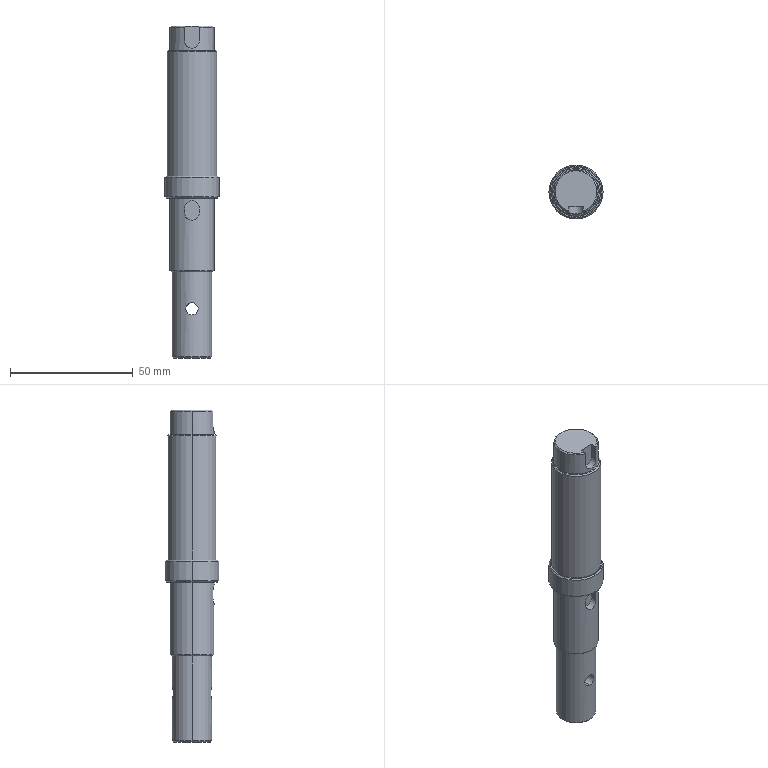Part | SolidWorks | features ICE 9, Chamfer 2, Extrusion 1 | 1 solid | 41 faces | box 22 x 22 x 135 mm | volume 36047 mm3 | cylinder 16 | cone 13 | plane 12 | commonest cylinder face diameters 6 x4 18 x4 5 x2 16 x2 20 x2 22 x2
STEP:
#1=CARTESIAN_POINT('',(0.,-8.,-52.));
#2=VERTEX_POINT('',#1);
#3=CARTESIAN_POINT('',(0.,-8.,-47.));
#4=VERTEX_POINT('',#3);
#5=CARTESIAN_POINT('',(0.,-8.,-52.));
#6=CARTESIAN_POINT('',(-0.1638,-8.,-52.));
#7=CARTESIAN_POINT('',(-0.3284,-7.995,-51.984));
#8=CARTESIAN_POINT('',(-0.6528,-7.975,-51.919));
#9=CARTESIAN_POINT('',(-0.8091,-7.96,-51.871));
#10=CARTESIAN_POINT('',(-1.111,-7.924,-51.746));
#11=CARTESIAN_POINT('',(-1.257,-7.902,-51.667));
#12=CARTESIAN_POINT('',(-1.527,-7.854,-51.486));
#13=CARTESIAN_POINT('',(-1.652,-7.828,-51.383));
#14=CARTESIAN_POINT('',(-1.883,-7.776,-51.152));
#15=CARTESIAN_POINT('',(-1.987,-7.75,-51.025));
#16=CARTESIAN_POINT('',(-2.168,-7.701,-50.756));
#17=CARTESIAN_POINT('',(-2.245,-7.679,-50.612));
#18=CARTESIAN_POINT('',(-2.372,-7.641,-50.308));
#19=CARTESIAN_POINT('',(-2.419,-7.626,-50.152));
#20=CARTESIAN_POINT('',(-2.483,-7.605,-49.831));
#21=CARTESIAN_POINT('',(-2.5,-7.599,-49.665));
#22=CARTESIAN_POINT('',(-2.5,-7.599,-49.335));
#23=CARTESIAN_POINT('',(-2.484,-7.605,-49.172));
#24=CARTESIAN_POINT('',(-2.42,-7.625,-48.85));
#25=CARTESIAN_POINT('',(-2.371,-7.641,-48.691));
#26=CARTESIAN_POINT('',(-2.183,-7.697,-48.239));
#27=CARTESIAN_POINT('',(-1.997,-7.75,-47.962));
#28=CARTESIAN_POINT('',(-1.654,-7.828,-47.618));
#29=CARTESIAN_POINT('',(-1.526,-7.854,-47.513));
#30=CARTESIAN_POINT('',(-1.256,-7.902,-47.332));
#31=CARTESIAN_POINT('',(-1.113,-7.924,-47.255));
#32=CARTESIAN_POINT('',(-0.8108,-7.96,-47.129));
#33=CARTESIAN_POINT('',(-0.6512,-7.975,-47.081));
#34=CARTESIAN_POINT('',(-0.3297,-7.995,-47.016));
#35=CARTESIAN_POINT('',(-0.1663,-8.,-47.));
#36=CARTESIAN_POINT('',(0.,-8.,-47.));
#37=B_SPLINE_CURVE_WITH_KNOTS('',3,(#5,#6,#7,#8,#9,#10,#11,#12,#13,#14,#15,#16,#17,#18,#19,#20,#21,#22,#23,#24,#25,#26,#27,#28,#29,#30,#31,#32,#33,#34,#35,#36),.UNSPECIFIED.,.F.,.F.,(4,2,2,2,2,2,2,2,2,2,2,2,2,2,2,4),(0.007866,0.008357,0.008849,0.00934,0.009832,0.01032,0.01081,0.01131,0.0118,0.01229,0.01278,0.01376,0.01425,0.01475,0.01524,0.01573),.UNSPECIFIED.);
#38=EDGE_CURVE('',#2,#4,#37,.T.);
#39=ORIENTED_EDGE('',*,*,#38,.F.);
#40=CARTESIAN_POINT('',(0.,8.,-52.));
#41=VERTEX_POINT('',#40);
#42=CARTESIAN_POINT('',(0.,-15.,-52.));
#43=DIRECTION('',(0.,1.,0.));
#44=VECTOR('',#43,1000.);
#45=LINE('',#42,#44);
#46=EDGE_CURVE('',#2,#41,#45,.T.);
#47=ORIENTED_EDGE('',*,*,#46,.T.);
#48=CARTESIAN_POINT('',(0.,8.,-47.));
#49=VERTEX_POINT('',#48);
#50=CARTESIAN_POINT('',(0.,8.,-47.));
#51=CARTESIAN_POINT('',(-0.1663,8.,-47.));
#52=CARTESIAN_POINT('',(-0.3296,7.995,-47.016));
#53=CARTESIAN_POINT('',(-0.6506,7.975,-47.081));
#54=CARTESIAN_POINT('',(-0.81,7.96,-47.129));
#55=CARTESIAN_POINT('',(-1.112,7.924,-47.255));
#56=CARTESIAN_POINT('',(-1.256,7.902,-47.332));
#57=CARTESIAN_POINT('',(-1.527,7.854,-47.513));
#58=CARTESIAN_POINT('',(-1.654,7.828,-47.618));
#59=CARTESIAN_POINT('',(-1.997,7.75,-47.962));
#60=CARTESIAN_POINT('',(-2.183,7.697,-48.239));
#61=CARTESIAN_POINT('',(-2.371,7.641,-48.69));
#62=CARTESIAN_POINT('',(-2.419,7.626,-48.848));
#63=CARTESIAN_POINT('',(-2.484,7.605,-49.172));
#64=CARTESIAN_POINT('',(-2.5,7.599,-49.335));
#65=CARTESIAN_POINT('',(-2.5,7.599,-49.663));
#66=CARTESIAN_POINT('',(-2.484,7.605,-49.83));
#67=CARTESIAN_POINT('',(-2.419,7.626,-50.151));
#68=CARTESIAN_POINT('',(-2.372,7.641,-50.308));
#69=CARTESIAN_POINT('',(-2.245,7.679,-50.612));
#70=CARTESIAN_POINT('',(-2.168,7.701,-50.756));
#71=CARTESIAN_POINT('',(-1.987,7.75,-51.026));
#72=CARTESIAN_POINT('',(-1.882,7.776,-51.153));
#73=CARTESIAN_POINT('',(-1.652,7.828,-51.384));
#74=CARTESIAN_POINT('',(-1.527,7.854,-51.486));
#75=CARTESIAN_POINT('',(-1.257,7.902,-51.667));
#76=CARTESIAN_POINT('',(-1.11,7.924,-51.746));
#77=CARTESIAN_POINT('',(-0.8089,7.96,-51.871));
#78=CARTESIAN_POINT('',(-0.6529,7.975,-51.919));
#79=CARTESIAN_POINT('',(-0.3297,7.995,-51.984));
#80=CARTESIAN_POINT('',(-0.1639,8.,-52.));
#81=CARTESIAN_POINT('',(0.,8.,-52.));
#82=B_SPLINE_CURVE_WITH_KNOTS('',3,(#50,#51,#52,#53,#54,#55,#56,#57,#58,#59,#60,#61,#62,#63,#64,#65,#66,#67,#68,#69,#70,#71,#72,#73,#74,#75,#76,#77,#78,#79,#80,#81),.UNSPECIFIED.,.F.,.F.,(4,2,2,2,2,2,2,2,2,2,2,2,2,2,2,4),(0.,0.0004916,0.0009832,0.001475,0.001966,0.00295,0.003441,0.003933,0.004424,0.004916,0.005408,0.005899,0.006391,0.006883,0.007374,0.007866),.UNSPECIFIED.);
#83=EDGE_CURVE('',#49,#41,#82,.T.);
#84=ORIENTED_EDGE('',*,*,#83,.F.);
#85=CARTESIAN_POINT('',(0.,-15.,-47.));
#86=DIRECTION('',(0.,1.,0.));
#87=VECTOR('',#86,1000.);
#88=LINE('',#85,#87);
#89=EDGE_CURVE('',#4,#49,#88,.T.);
#90=ORIENTED_EDGE('',*,*,#89,.F.);
#91=EDGE_LOOP('',(#39,#47,#84,#90));
#92=FACE_OUTER_BOUND('',#91,.T.);
#93=CARTESIAN_POINT('',(0.,-15.,-49.5));
#94=DIRECTION('',(0.,1.,0.));
#95=DIRECTION('',(0.,0.,1.));
#96=AXIS2_PLACEMENT_3D('',#93,#94,#95);
#97=CYLINDRICAL_SURFACE('',#96,2.5);
#98=ADVANCED_FACE('',(#92),#97,.F.);
#99=CARTESIAN_POINT('',(-7.5,0.,-69.5));
#100=VERTEX_POINT('',#99);
#101=CARTESIAN_POINT('',(7.5,0.,-69.5));
#102=VERTEX_POINT('',#101);
#103=CARTESIAN_POINT('',(0.,0.,-69.5));
#104=DIRECTION('',(0.,0.,-1.));
#105=DIRECTION('',(-1.,0.,0.));
#106=AXIS2_PLACEMENT_3D('',#103,#104,#105);
#107=CIRCLE('',#106,7.5);
#108=EDGE_CURVE('',#100,#102,#107,.T.);
#109=ORIENTED_EDGE('',*,*,#108,.F.);
#110=CARTESIAN_POINT('',(-8.,0.,-69.));
#111=VERTEX_POINT('',#110);
#112=CARTESIAN_POINT('',(-7.5,0.,-69.5));
#113=DIRECTION('',(-0.7071,0.,0.7071));
#114=VECTOR('',#113,1000.);
#115=LINE('',#112,#114);
#116=EDGE_CURVE('',#100,#111,#115,.T.);
#117=ORIENTED_EDGE('',*,*,#116,.T.);
#118=CARTESIAN_POINT('',(8.,0.,-69.));
#119=VERTEX_POINT('',#118);
#120=CARTESIAN_POINT('',(0.,0.,-69.));
#121=DIRECTION('',(0.,0.,1.));
#122=DIRECTION('',(-1.,0.,0.));
#123=AXIS2_PLACEMENT_3D('',#120,#121,#122);
#124=CIRCLE('',#123,8.);
#125=EDGE_CURVE('',#119,#111,#124,.T.);
#126=ORIENTED_EDGE('',*,*,#125,.F.);
#127=CARTESIAN_POINT('',(7.5,0.,-69.5));
#128=DIRECTION('',(0.7071,0.,0.7071));
#129=VECTOR('',#128,1000.);
#130=LINE('',#127,#129);
#131=EDGE_CURVE('',#102,#119,#130,.T.);
#132=ORIENTED_EDGE('',*,*,#131,.F.);
#133=EDGE_LOOP('',(#109,#117,#126,#132));
#134=FACE_OUTER_BOUND('',#133,.T.);
#135=CARTESIAN_POINT('',(0.,0.,-69.5));
#136=DIRECTION('',(0.,0.,1.));
#137=DIRECTION('',(1.,0.,0.));
#138=AXIS2_PLACEMENT_3D('',#135,#136,#137);
#139=CONICAL_SURFACE('',#138,7.5,0.7854);
#140=ADVANCED_FACE('',(#134),#139,.T.);
#141=ORIENTED_EDGE('',*,*,#83,.T.);
#142=CARTESIAN_POINT('',(0.,8.,-52.));
#143=CARTESIAN_POINT('',(0.1638,8.,-52.));
#144=CARTESIAN_POINT('',(0.3284,7.995,-51.984));
#145=CARTESIAN_POINT('',(0.6528,7.975,-51.919));
#146=CARTESIAN_POINT('',(0.8091,7.96,-51.871));
#147=CARTESIAN_POINT('',(1.111,7.924,-51.746));
#148=CARTESIAN_POINT('',(1.257,7.902,-51.667));
#149=CARTESIAN_POINT('',(1.527,7.854,-51.486));
#150=CARTESIAN_POINT('',(1.652,7.828,-51.383));
#151=CARTESIAN_POINT('',(1.883,7.776,-51.152));
#152=CARTESIAN_POINT('',(1.987,7.75,-51.025));
#153=CARTESIAN_POINT('',(2.168,7.701,-50.756));
#154=CARTESIAN_POINT('',(2.245,7.679,-50.612));
#155=CARTESIAN_POINT('',(2.372,7.641,-50.308));
#156=CARTESIAN_POINT('',(2.419,7.626,-50.152));
#157=CARTESIAN_POINT('',(2.483,7.605,-49.831));
#158=CARTESIAN_POINT('',(2.5,7.599,-49.665));
#159=CARTESIAN_POINT('',(2.5,7.599,-49.335));
#160=CARTESIAN_POINT('',(2.484,7.605,-49.172));
#161=CARTESIAN_POINT('',(2.42,7.625,-48.85));
#162=CARTESIAN_POINT('',(2.371,7.641,-48.691));
#163=CARTESIAN_POINT('',(2.183,7.697,-48.239));
#164=CARTESIAN_POINT('',(1.997,7.75,-47.962));
#165=CARTESIAN_POINT('',(1.654,7.828,-47.618));
#166=CARTESIAN_POINT('',(1.526,7.854,-47.513));
#167=CARTESIAN_POINT('',(1.256,7.902,-47.332));
#168=CARTESIAN_POINT('',(1.113,7.924,-47.255));
#169=CARTESIAN_POINT('',(0.8108,7.96,-47.129));
#170=CARTESIAN_POINT('',(0.6512,7.975,-47.081));
#171=CARTESIAN_POINT('',(0.3297,7.995,-47.016));
#172=CARTESIAN_POINT('',(0.1663,8.,-47.));
#173=CARTESIAN_POINT('',(0.,8.,-47.));
#174=B_SPLINE_CURVE_WITH_KNOTS('',3,(#142,#143,#144,#145,#146,#147,#148,#149,#150,#151,#152,#153,#154,#155,#156,#157,#158,#159,#160,#161,#162,#163,#164,#165,#166,#167,#168,#169,#170,#171,#172,#173),.UNSPECIFIED.,.F.,.F.,(4,2,2,2,2,2,2,2,2,2,2,2,2,2,2,4),(0.007866,0.008357,0.008849,0.00934,0.009832,0.01032,0.01081,0.01131,0.0118,0.01229,0.01278,0.01376,0.01425,0.01475,0.01524,0.01573),.UNSPECIFIED.);
#175=EDGE_CURVE('',#41,#49,#174,.T.);
#176=ORIENTED_EDGE('',*,*,#175,.T.);
#177=EDGE_LOOP('',(#141,#176));
#178=FACE_BOUND('',#177,.T.);
#179=ORIENTED_EDGE('',*,*,#125,.T.);
#180=CARTESIAN_POINT('',(-8.,0.,-34.5));
#181=VERTEX_POINT('',#180);
#182=CARTESIAN_POINT('',(-8.,0.,-69.5));
#183=DIRECTION('',(0.,0.,1.));
#184=VECTOR('',#183,1000.);
#185=LINE('',#182,#184);
#186=EDGE_CURVE('',#111,#181,#185,.T.);
#187=ORIENTED_EDGE('',*,*,#186,.T.);
#188=CARTESIAN_POINT('',(8.,0.,-34.5));
#189=VERTEX_POINT('',#188);
#190=CARTESIAN_POINT('',(0.,0.,-34.5));
#191=DIRECTION('',(0.,0.,-1.));
#192=DIRECTION('',(-1.,0.,0.));
#193=AXIS2_PLACEMENT_3D('',#190,#191,#192);
#194=CIRCLE('',#193,8.);
#195=EDGE_CURVE('',#181,#189,#194,.T.);
#196=ORIENTED_EDGE('',*,*,#195,.T.);
#197=CARTESIAN_POINT('',(8.,0.,-69.5));
#198=DIRECTION('',(0.,0.,1.));
#199=VECTOR('',#198,1000.);
#200=LINE('',#197,#199);
#201=EDGE_CURVE('',#119,#189,#200,.T.);
#202=ORIENTED_EDGE('',*,*,#201,.F.);
#203=EDGE_LOOP('',(#179,#187,#196,#202));
#204=FACE_OUTER_BOUND('',#203,.T.);
#205=CARTESIAN_POINT('',(0.,0.,-69.5));
#206=DIRECTION('',(0.,0.,1.));
#207=DIRECTION('',(1.,0.,0.));
#208=AXIS2_PLACEMENT_3D('',#205,#206,#207);
#209=CYLINDRICAL_SURFACE('',#208,8.);
#210=ADVANCED_FACE('',(#178,#204),#209,.T.);
#211=CARTESIAN_POINT('',(8.5,0.,65.5));
#212=VERTEX_POINT('',#211);
#213=CARTESIAN_POINT('',(-8.5,0.,65.5));
#214=VERTEX_POINT('',#213);
#215=CARTESIAN_POINT('',(0.,0.,65.5));
#216=DIRECTION('',(0.,0.,1.));
#217=DIRECTION('',(1.,0.,0.));
#218=AXIS2_PLACEMENT_3D('',#215,#216,#217);
#219=CIRCLE('',#218,8.5);
#220=EDGE_CURVE('',#212,#214,#219,.T.);
#221=ORIENTED_EDGE('',*,*,#220,.F.);
#222=CARTESIAN_POINT('',(9.,0.,65.));
#223=VERTEX_POINT('',#222);
#224=CARTESIAN_POINT('',(8.5,0.,65.5));
#225=DIRECTION('',(0.7071,0.,-0.7071));
#226=VECTOR('',#225,1000.);
#227=LINE('',#224,#226);
#228=EDGE_CURVE('',#212,#223,#227,.T.);
#229=ORIENTED_EDGE('',*,*,#228,.T.);
#230=CARTESIAN_POINT('',(-9.,0.,65.));
#231=VERTEX_POINT('',#230);
#232=CARTESIAN_POINT('',(0.,0.,65.));
#233=DIRECTION('',(0.,0.,-1.));
#234=DIRECTION('',(1.,0.,0.));
#235=AXIS2_PLACEMENT_3D('',#232,#233,#234);
#236=CIRCLE('',#235,9.);
#237=EDGE_CURVE('',#231,#223,#236,.T.);
#238=ORIENTED_EDGE('',*,*,#237,.F.);
#239=CARTESIAN_POINT('',(-8.5,0.,65.5));
#240=DIRECTION('',(-0.7071,0.,-0.7071));
#241=VECTOR('',#240,1000.);
#242=LINE('',#239,#241);
#243=EDGE_CURVE('',#214,#231,#242,.T.);
#244=ORIENTED_EDGE('',*,*,#243,.F.);
#245=EDGE_LOOP('',(#221,#229,#238,#244));
#246=FACE_OUTER_BOUND('',#245,.T.);
#247=CARTESIAN_POINT('',(0.,0.,65.5));
#248=DIRECTION('',(0.,0.,-1.));
#249=DIRECTION('',(-1.,0.,0.));
#250=AXIS2_PLACEMENT_3D('',#247,#248,#249);
#251=CONICAL_SURFACE('',#250,8.5,0.7854);
#252=ADVANCED_FACE('',(#246),#251,.T.);
#253=CARTESIAN_POINT('',(-3.,-7.953,65.5));
#254=VERTEX_POINT('',#253);
#255=CARTESIAN_POINT('',(0.,0.,65.5));
#256=DIRECTION('',(0.,0.,1.));
#257=DIRECTION('',(1.,0.,0.));
#258=AXIS2_PLACEMENT_3D('',#255,#256,#257);
#259=CIRCLE('',#258,8.5);
#260=EDGE_CURVE('',#214,#254,#259,.T.);
#261=ORIENTED_EDGE('',*,*,#260,.F.);
#262=ORIENTED_EDGE('',*,*,#243,.T.);
#263=CARTESIAN_POINT('',(-3.,-8.485,65.));
#264=VERTEX_POINT('',#263);
#265=CARTESIAN_POINT('',(0.,0.,65.));
#266=DIRECTION('',(0.,0.,-1.));
#267=DIRECTION('',(1.,0.,0.));
#268=AXIS2_PLACEMENT_3D('',#265,#266,#267);
#269=CIRCLE('',#268,9.);
#270=EDGE_CURVE('',#264,#231,#269,.T.);
#271=ORIENTED_EDGE('',*,*,#270,.F.);
#272=CARTESIAN_POINT('',(-3.,-7.953,65.5));
#273=CARTESIAN_POINT('',(-3.,-8.131,65.334));
#274=CARTESIAN_POINT('',(-3.,-8.308,65.167));
#275=CARTESIAN_POINT('',(-3.,-8.485,65.));
#276=B_SPLINE_CURVE_WITH_KNOTS('',3,(#272,#273,#274,#275),.UNSPECIFIED.,.F.,.F.,(4,4),(0.,0.0007303),.UNSPECIFIED.);
#277=EDGE_CURVE('',#254,#264,#276,.T.);
#278=ORIENTED_EDGE('',*,*,#277,.F.);
#279=EDGE_LOOP('',(#261,#262,#271,#278));
#280=FACE_OUTER_BOUND('',#279,.T.);
#281=CARTESIAN_POINT('',(0.,0.,65.5));
#282=DIRECTION('',(0.,0.,-1.));
#283=DIRECTION('',(-1.,0.,0.));
#284=AXIS2_PLACEMENT_3D('',#281,#282,#283);
#285=CONICAL_SURFACE('',#284,8.5,0.7854);
#286=ADVANCED_FACE('',(#280),#285,.T.);
#287=CARTESIAN_POINT('',(9.5,0.,55.5));
#288=VERTEX_POINT('',#287);
#289=CARTESIAN_POINT('',(-9.5,0.,55.5));
#290=VERTEX_POINT('',#289);
#291=CARTESIAN_POINT('',(0.,0.,55.5));
#292=DIRECTION('',(0.,0.,1.));
#293=DIRECTION('',(1.,0.,0.));
#294=AXIS2_PLACEMENT_3D('',#291,#292,#293);
#295=CIRCLE('',#294,9.5);
#296=EDGE_CURVE('',#288,#290,#295,.T.);
#297=ORIENTED_EDGE('',*,*,#296,.F.);
#298=CARTESIAN_POINT('',(10.,0.,55.));
#299=VERTEX_POINT('',#298);
#300=CARTESIAN_POINT('',(9.5,0.,55.5));
#301=DIRECTION('',(0.7071,0.,-0.7071));
#302=VECTOR('',#301,1000.);
#303=LINE('',#300,#302);
#304=EDGE_CURVE('',#288,#299,#303,.T.);
#305=ORIENTED_EDGE('',*,*,#304,.T.);
#306=CARTESIAN_POINT('',(-10.,0.,55.));
#307=VERTEX_POINT('',#306);
#308=CARTESIAN_POINT('',(0.,0.,55.));
#309=DIRECTION('',(0.,0.,-1.));
#310=DIRECTION('',(1.,0.,0.));
#311=AXIS2_PLACEMENT_3D('',#308,#309,#310);
#312=CIRCLE('',#311,10.);
#313=EDGE_CURVE('',#307,#299,#312,.T.);
#314=ORIENTED_EDGE('',*,*,#313,.F.);
#315=CARTESIAN_POINT('',(-9.5,0.,55.5));
#316=DIRECTION('',(-0.7071,0.,-0.7071));
#317=VECTOR('',#316,1000.);
#318=LINE('',#315,#317);
#319=EDGE_CURVE('',#290,#307,#318,.T.);
#320=ORIENTED_EDGE('',*,*,#319,.F.);
#321=EDGE_LOOP('',(#297,#305,#314,#320));
#322=FACE_OUTER_BOUND('',#321,.T.);
#323=CARTESIAN_POINT('',(0.,0.,55.5));
#324=DIRECTION('',(0.,0.,-1.));
#325=DIRECTION('',(-1.,0.,0.));
#326=AXIS2_PLACEMENT_3D('',#323,#324,#325);
#327=CONICAL_SURFACE('',#326,9.5,0.7854);
#328=ADVANCED_FACE('',(#322),#327,.T.);
#329=CARTESIAN_POINT('',(10.5,0.,4.5));
#330=VERTEX_POINT('',#329);
#331=CARTESIAN_POINT('',(-10.5,0.,4.5));
#332=VERTEX_POINT('',#331);
#333=CARTESIAN_POINT('',(0.,0.,4.5));
#334=DIRECTION('',(0.,0.,1.));
#335=DIRECTION('',(1.,0.,0.));
#336=AXIS2_PLACEMENT_3D('',#333,#334,#335);
#337=CIRCLE('',#336,10.5);
#338=EDGE_CURVE('',#330,#332,#337,.T.);
#339=ORIENTED_EDGE('',*,*,#338,.F.);
#340=CARTESIAN_POINT('',(11.,0.,4.));
#341=VERTEX_POINT('',#340);
#342=CARTESIAN_POINT('',(10.5,0.,4.5));
#343=DIRECTION('',(0.7071,0.,-0.7071));
#344=VECTOR('',#343,1000.);
#345=LINE('',#342,#344);
#346=EDGE_CURVE('',#330,#341,#345,.T.);
#347=ORIENTED_EDGE('',*,*,#346,.T.);
#348=CARTESIAN_POINT('',(-11.,0.,4.));
#349=VERTEX_POINT('',#348);
#350=CARTESIAN_POINT('',(0.,0.,4.));
#351=DIRECTION('',(0.,0.,-1.));
#352=DIRECTION('',(1.,0.,0.));
#353=AXIS2_PLACEMENT_3D('',#350,#351,#352);
#354=CIRCLE('',#353,11.);
#355=EDGE_CURVE('',#349,#341,#354,.T.);
#356=ORIENTED_EDGE('',*,*,#355,.F.);
#357=CARTESIAN_POINT('',(-10.5,0.,4.5));
#358=DIRECTION('',(-0.7071,0.,-0.7071));
#359=VECTOR('',#358,1000.);
#360=LINE('',#357,#359);
#361=EDGE_CURVE('',#332,#349,#360,.T.);
#362=ORIENTED_EDGE('',*,*,#361,.F.);
#363=EDGE_LOOP('',(#339,#347,#356,#362));
#364=FACE_OUTER_BOUND('',#363,.T.);
#365=CARTESIAN_POINT('',(0.,0.,4.5));
#366=DIRECTION('',(0.,0.,-1.));
#367=DIRECTION('',(-1.,0.,0.));
#368=AXIS2_PLACEMENT_3D('',#365,#366,#367);
#369=CONICAL_SURFACE('',#368,10.5,0.7854);
#370=ADVANCED_FACE('',(#364),#369,.T.);
#371=CARTESIAN_POINT('',(-10.5,0.,-4.5));
#372=VERTEX_POINT('',#371);
#373=CARTESIAN_POINT('',(10.5,0.,-4.5));
#374=VERTEX_POINT('',#373);
#375=CARTESIAN_POINT('',(0.,0.,-4.5));
#376=DIRECTION('',(0.,0.,-1.));
#377=DIRECTION('',(1.,0.,0.));
#378=AXIS2_PLACEMENT_3D('',#375,#376,#377);
#379=CIRCLE('',#378,10.5);
#380=EDGE_CURVE('',#372,#374,#379,.T.);
#381=ORIENTED_EDGE('',*,*,#380,.F.);
#382=CARTESIAN_POINT('',(-11.,0.,-4.));
#383=VERTEX_POINT('',#382);
#384=CARTESIAN_POINT('',(-11.,0.,-4.));
#385=DIRECTION('',(-0.7071,0.,0.7071));
#386=VECTOR('',#385,1000.);
#387=LINE('',#384,#386);
#388=EDGE_CURVE('',#372,#383,#387,.T.);
#389=ORIENTED_EDGE('',*,*,#388,.T.);
#390=CARTESIAN_POINT('',(11.,0.,-4.));
#391=VERTEX_POINT('',#390);
#392=CARTESIAN_POINT('',(0.,0.,-4.));
#393=DIRECTION('',(0.,0.,1.));
#394=DIRECTION('',(1.,0.,0.));
#395=AXIS2_PLACEMENT_3D('',#392,#393,#394);
#396=CIRCLE('',#395,11.);
#397=EDGE_CURVE('',#391,#383,#396,.T.);
#398=ORIENTED_EDGE('',*,*,#397,.F.);
#399=CARTESIAN_POINT('',(11.,0.,-4.));
#400=DIRECTION('',(0.7071,0.,0.7071));
#401=VECTOR('',#400,1000.);
#402=LINE('',#399,#401);
#403=EDGE_CURVE('',#374,#391,#402,.T.);
#404=ORIENTED_EDGE('',*,*,#403,.F.);
#405=EDGE_LOOP('',(#381,#389,#398,#404));
#406=FACE_OUTER_BOUND('',#405,.T.);
#407=CARTESIAN_POINT('',(0.,0.,-4.));
#408=DIRECTION('',(0.,0.,1.));
#409=DIRECTION('',(1.,0.,0.));
#410=AXIS2_PLACEMENT_3D('',#407,#408,#409);
#411=CONICAL_SURFACE('',#410,11.,0.7854);
#412=ADVANCED_FACE('',(#406),#411,.T.);
#413=CARTESIAN_POINT('',(-8.5,0.,-34.5));
#414=VERTEX_POINT('',#413);
#415=CARTESIAN_POINT('',(8.5,0.,-34.5));
#416=VERTEX_POINT('',#415);
#417=CARTESIAN_POINT('',(0.,0.,-34.5));
#418=DIRECTION('',(0.,0.,-1.));
#419=DIRECTION('',(-1.,0.,0.));
#420=AXIS2_PLACEMENT_3D('',#417,#418,#419);
#421=CIRCLE('',#420,8.5);
#422=EDGE_CURVE('',#414,#416,#421,.T.);
#423=ORIENTED_EDGE('',*,*,#422,.F.);
#424=CARTESIAN_POINT('',(-9.,0.,-34.));
#425=VERTEX_POINT('',#424);
#426=CARTESIAN_POINT('',(-8.5,0.,-34.5));
#427=DIRECTION('',(-0.7071,0.,0.7071));
#428=VECTOR('',#427,1000.);
#429=LINE('',#426,#428);
#430=EDGE_CURVE('',#414,#425,#429,.T.);
#431=ORIENTED_EDGE('',*,*,#430,.T.);
#432=CARTESIAN_POINT('',(9.,0.,-34.));
#433=VERTEX_POINT('',#432);
#434=CARTESIAN_POINT('',(0.,0.,-34.));
#435=DIRECTION('',(0.,0.,1.));
#436=DIRECTION('',(-1.,0.,0.));
#437=AXIS2_PLACEMENT_3D('',#434,#435,#436);
#438=CIRCLE('',#437,9.);
#439=EDGE_CURVE('',#433,#425,#438,.T.);
#440=ORIENTED_EDGE('',*,*,#439,.F.);
#441=CARTESIAN_POINT('',(8.5,0.,-34.5));
#442=DIRECTION('',(0.7071,0.,0.7071));
#443=VECTOR('',#442,1000.);
#444=LINE('',#441,#443);
#445=EDGE_CURVE('',#416,#433,#444,.T.);
#446=ORIENTED_EDGE('',*,*,#445,.F.);
#447=EDGE_LOOP('',(#423,#431,#440,#446));
#448=FACE_OUTER_BOUND('',#447,.T.);
#449=CARTESIAN_POINT('',(0.,0.,-34.5));
#450=DIRECTION('',(0.,0.,1.));
#451=DIRECTION('',(1.,0.,0.));
#452=AXIS2_PLACEMENT_3D('',#449,#450,#451);
#453=CONICAL_SURFACE('',#452,8.5,0.7854);
#454=ADVANCED_FACE('',(#448),#453,.T.);
#455=CARTESIAN_POINT('',(0.,-9.,-5.5));
#456=VERTEX_POINT('',#455);
#457=CARTESIAN_POINT('',(3.,-8.485,-8.5));
#458=VERTEX_POINT('',#457);
#459=CARTESIAN_POINT('',(0.,-9.,-5.5));
#460=CARTESIAN_POINT('',(0.1971,-9.,-5.5));
#461=CARTESIAN_POINT('',(0.3973,-8.993,-5.52));
#462=CARTESIAN_POINT('',(0.7829,-8.968,-5.597));
#463=CARTESIAN_POINT('',(0.9705,-8.949,-5.654));
#464=CARTESIAN_POINT('',(1.335,-8.902,-5.806));
#465=CARTESIAN_POINT('',(1.508,-8.874,-5.899));
#466=CARTESIAN_POINT('',(1.831,-8.813,-6.116));
#467=CARTESIAN_POINT('',(1.984,-8.78,-6.241));
#468=CARTESIAN_POINT('',(2.26,-8.713,-6.517));
#469=CARTESIAN_POINT('',(2.383,-8.68,-6.667));
#470=CARTESIAN_POINT('',(2.6,-8.617,-6.991));
#471=CARTESIAN_POINT('',(2.694,-8.588,-7.166));
#472=CARTESIAN_POINT('',(2.844,-8.539,-7.526));
#473=CARTESIAN_POINT('',(2.902,-8.519,-7.713));
#474=CARTESIAN_POINT('',(2.98,-8.492,-8.101));
#475=CARTESIAN_POINT('',(3.,-8.485,-8.3));
#476=CARTESIAN_POINT('',(3.,-8.485,-8.5));
#477=B_SPLINE_CURVE_WITH_KNOTS('',3,(#459,#460,#461,#462,#463,#464,#465,#466,#467,#468,#469,#470,#471,#472,#473,#474,#475,#476),.UNSPECIFIED.,.F.,.F.,(4,2,2,2,2,2,2,2,4),(0.004725,0.005315,0.005905,0.006494,0.007084,0.007674,0.008264,0.008854,0.009444),.UNSPECIFIED.);
#478=EDGE_CURVE('',#456,#458,#477,.T.);
#479=ORIENTED_EDGE('',*,*,#478,.F.);
#480=CARTESIAN_POINT('',(0.,-6.,-5.5));
#481=VERTEX_POINT('',#480);
#482=CARTESIAN_POINT('',(0.,-19.,-5.5));
#483=DIRECTION('',(0.,1.,0.));
#484=VECTOR('',#483,1000.);
#485=LINE('',#482,#484);
#486=EDGE_CURVE('',#456,#481,#485,.T.);
#487=ORIENTED_EDGE('',*,*,#486,.T.);
#488=CARTESIAN_POINT('',(3.,-6.,-8.5));
#489=VERTEX_POINT('',#488);
#490=CARTESIAN_POINT('',(0.,-6.,-8.5));
#491=DIRECTION('',(0.,-1.,0.));
#492=DIRECTION('',(0.,0.,-1.));
#493=AXIS2_PLACEMENT_3D('',#490,#491,#492);
#494=CIRCLE('',#493,3.);
#495=EDGE_CURVE('',#489,#481,#494,.T.);
#496=ORIENTED_EDGE('',*,*,#495,.F.);
#497=CARTESIAN_POINT('',(3.,-19.,-8.5));
#498=DIRECTION('',(0.,1.,0.));
#499=VECTOR('',#498,1000.);
#500=LINE('',#497,#499);
#501=EDGE_CURVE('',#458,#489,#500,.T.);
#502=ORIENTED_EDGE('',*,*,#501,.F.);
#503=EDGE_LOOP('',(#479,#487,#496,#502));
#504=FACE_OUTER_BOUND('',#503,.T.);
#505=CARTESIAN_POINT('',(0.,-19.,-8.5));
#506=DIRECTION('',(0.,1.,0.));
#507=DIRECTION('',(0.,0.,1.));
#508=AXIS2_PLACEMENT_3D('',#505,#506,#507);
#509=CYLINDRICAL_SURFACE('',#508,3.);
#510=ADVANCED_FACE('',(#504),#509,.F.);
#511=ORIENTED_EDGE('',*,*,#237,.T.);
#512=CARTESIAN_POINT('',(9.,0.,55.5));
#513=VERTEX_POINT('',#512);
#514=CARTESIAN_POINT('',(9.,0.,65.5));
#515=DIRECTION('',(0.,0.,-1.));
#516=VECTOR('',#515,1000.);
#517=LINE('',#514,#516);
#518=EDGE_CURVE('',#223,#513,#517,.T.);
#519=ORIENTED_EDGE('',*,*,#518,.T.);
#520=CARTESIAN_POINT('',(-9.,0.,55.5));
#521=VERTEX_POINT('',#520);
#522=CARTESIAN_POINT('',(0.,0.,55.5));
#523=DIRECTION('',(0.,0.,1.));
#524=DIRECTION('',(1.,0.,0.));
#525=AXIS2_PLACEMENT_3D('',#522,#523,#524);
#526=CIRCLE('',#525,9.);
#527=EDGE_CURVE('',#513,#521,#526,.T.);
#528=ORIENTED_EDGE('',*,*,#527,.T.);
#529=CARTESIAN_POINT('',(-9.,0.,65.5));
#530=DIRECTION('',(0.,0.,-1.));
#531=VECTOR('',#530,1000.);
#532=LINE('',#529,#531);
#533=EDGE_CURVE('',#231,#521,#532,.T.);
#534=ORIENTED_EDGE('',*,*,#533,.F.);
#535=EDGE_LOOP('',(#511,#519,#528,#534));
#536=FACE_OUTER_BOUND('',#535,.T.);
#537=CARTESIAN_POINT('',(0.,0.,65.5));
#538=DIRECTION('',(0.,0.,-1.));
#539=DIRECTION('',(-1.,0.,0.));
#540=AXIS2_PLACEMENT_3D('',#537,#538,#539);
#541=CYLINDRICAL_SURFACE('',#540,9.);
#542=ADVANCED_FACE('',(#536),#541,.T.);
#543=ORIENTED_EDGE('',*,*,#313,.T.);
#544=CARTESIAN_POINT('',(10.,0.,4.5));
#545=VERTEX_POINT('',#544);
#546=CARTESIAN_POINT('',(10.,0.,55.5));
#547=DIRECTION('',(0.,0.,-1.));
#548=VECTOR('',#547,1000.);
#549=LINE('',#546,#548);
#550=EDGE_CURVE('',#299,#545,#549,.T.);
#551=ORIENTED_EDGE('',*,*,#550,.T.);
#552=CARTESIAN_POINT('',(-10.,0.,4.5));
#553=VERTEX_POINT('',#552);
#554=CARTESIAN_POINT('',(0.,0.,4.5));
#555=DIRECTION('',(0.,0.,1.));
#556=DIRECTION('',(1.,0.,0.));
#557=AXIS2_PLACEMENT_3D('',#554,#555,#556);
#558=CIRCLE('',#557,10.);
#559=EDGE_CURVE('',#545,#553,#558,.T.);
#560=ORIENTED_EDGE('',*,*,#559,.T.);
#561=CARTESIAN_POINT('',(-10.,0.,55.5));
#562=DIRECTION('',(0.,0.,-1.));
#563=VECTOR('',#562,1000.);
#564=LINE('',#561,#563);
#565=EDGE_CURVE('',#307,#553,#564,.T.);
#566=ORIENTED_EDGE('',*,*,#565,.F.);
#567=EDGE_LOOP('',(#543,#551,#560,#566));
#568=FACE_OUTER_BOUND('',#567,.T.);
#569=CARTESIAN_POINT('',(0.,0.,55.5));
#570=DIRECTION('',(0.,0.,-1.));
#571=DIRECTION('',(-1.,0.,0.));
#572=AXIS2_PLACEMENT_3D('',#569,#570,#571);
#573=CYLINDRICAL_SURFACE('',#572,10.);
#574=ADVANCED_FACE('',(#568),#573,.T.);
#575=ORIENTED_EDGE('',*,*,#439,.T.);
#576=CARTESIAN_POINT('',(-9.,0.,-4.5));
#577=VERTEX_POINT('',#576);
#578=CARTESIAN_POINT('',(-9.,0.,-34.5));
#579=DIRECTION('',(0.,0.,1.));
#580=VECTOR('',#579,1000.);
#581=LINE('',#578,#580);
#582=EDGE_CURVE('',#425,#577,#581,.T.);
#583=ORIENTED_EDGE('',*,*,#582,.T.);
#584=CARTESIAN_POINT('',(9.,0.,-4.5));
#585=VERTEX_POINT('',#584);
#586=CARTESIAN_POINT('',(0.,0.,-4.5));
#587=DIRECTION('',(0.,0.,-1.));
#588=DIRECTION('',(1.,0.,0.));
#589=AXIS2_PLACEMENT_3D('',#586,#587,#588);
#590=CIRCLE('',#589,9.);
#591=EDGE_CURVE('',#577,#585,#590,.T.);
#592=ORIENTED_EDGE('',*,*,#591,.T.);
#593=CARTESIAN_POINT('',(9.,0.,-34.5));
#594=DIRECTION('',(0.,0.,1.));
#595=VECTOR('',#594,1000.);
#596=LINE('',#593,#595);
#597=EDGE_CURVE('',#433,#585,#596,.T.);
#598=ORIENTED_EDGE('',*,*,#597,.F.);
#599=EDGE_LOOP('',(#575,#583,#592,#598));
#600=FACE_OUTER_BOUND('',#599,.T.);
#601=CARTESIAN_POINT('',(0.,0.,-34.5));
#602=DIRECTION('',(0.,0.,1.));
#603=DIRECTION('',(1.,0.,0.));
#604=AXIS2_PLACEMENT_3D('',#601,#602,#603);
#605=CYLINDRICAL_SURFACE('',#604,9.);
#606=ADVANCED_FACE('',(#600),#605,.T.);
#607=ORIENTED_EDGE('',*,*,#355,.T.);
#608=CARTESIAN_POINT('',(11.,0.,4.5));
#609=DIRECTION('',(0.,0.,-1.));
#610=VECTOR('',#609,1000.);
#611=LINE('',#608,#610);
#612=EDGE_CURVE('',#341,#391,#611,.T.);
#613=ORIENTED_EDGE('',*,*,#612,.T.);
#614=ORIENTED_EDGE('',*,*,#397,.T.);
#615=CARTESIAN_POINT('',(-11.,0.,4.5));
#616=DIRECTION('',(0.,0.,-1.));
#617=VECTOR('',#616,1000.);
#618=LINE('',#615,#617);
#619=EDGE_CURVE('',#349,#383,#618,.T.);
#620=ORIENTED_EDGE('',*,*,#619,.F.);
#621=EDGE_LOOP('',(#607,#613,#614,#620));
#622=FACE_OUTER_BOUND('',#621,.T.);
#623=CARTESIAN_POINT('',(0.,0.,4.5));
#624=DIRECTION('',(0.,0.,-1.));
#625=DIRECTION('',(-1.,0.,0.));
#626=AXIS2_PLACEMENT_3D('',#623,#624,#625);
#627=CYLINDRICAL_SURFACE('',#626,11.);
#628=ADVANCED_FACE('',(#622),#627,.T.);
#629=CARTESIAN_POINT('',(0.,0.,-34.5));
#630=DIRECTION('',(0.,0.,-1.));
#631=DIRECTION('',(-1.,0.,0.));
#632=AXIS2_PLACEMENT_3D('',#629,#630,#631);
#633=CIRCLE('',#632,8.5);
#634=EDGE_CURVE('',#416,#414,#633,.T.);
#635=ORIENTED_EDGE('',*,*,#634,.T.);
#636=ORIENTED_EDGE('',*,*,#422,.T.);
#637=EDGE_LOOP('',(#635,#636));
#638=FACE_OUTER_BOUND('',#637,.T.);
#639=CARTESIAN_POINT('',(0.,0.,-34.5));
#640=DIRECTION('',(0.,0.,-1.));
#641=DIRECTION('',(-1.,0.,0.));
#642=AXIS2_PLACEMENT_3D('',#639,#640,#641);
#643=CIRCLE('',#642,8.);
#644=EDGE_CURVE('',#189,#181,#643,.T.);
#645=ORIENTED_EDGE('',*,*,#644,.F.);
#646=ORIENTED_EDGE('',*,*,#195,.F.);
#647=EDGE_LOOP('',(#645,#646));
#648=FACE_BOUND('',#647,.T.);
#649=CARTESIAN_POINT('',(0.,0.,-34.5));
#650=DIRECTION('',(0.,0.,-1.));
#651=DIRECTION('',(-1.,0.,0.));
#652=AXIS2_PLACEMENT_3D('',#649,#650,#651);
#653=PLANE('',#652);
#654=ADVANCED_FACE('',(#638,#648),#653,.T.);
#655=CARTESIAN_POINT('',(0.,0.,55.5));
#656=DIRECTION('',(0.,0.,1.));
#657=DIRECTION('',(1.,0.,0.));
#658=AXIS2_PLACEMENT_3D('',#655,#656,#657);
#659=CIRCLE('',#658,9.5);
#660=EDGE_CURVE('',#290,#288,#659,.T.);
#661=ORIENTED_EDGE('',*,*,#660,.T.);
#662=ORIENTED_EDGE('',*,*,#296,.T.);
#663=EDGE_LOOP('',(#661,#662));
#664=FACE_OUTER_BOUND('',#663,.T.);
#665=CARTESIAN_POINT('',(0.,0.,55.5));
#666=DIRECTION('',(0.,0.,1.));
#667=DIRECTION('',(1.,0.,0.));
#668=AXIS2_PLACEMENT_3D('',#665,#666,#667);
#669=CIRCLE('',#668,9.);
#670=EDGE_CURVE('',#521,#513,#669,.T.);
#671=ORIENTED_EDGE('',*,*,#670,.F.);
#672=ORIENTED_EDGE('',*,*,#527,.F.);
#673=EDGE_LOOP('',(#671,#672));
#674=FACE_BOUND('',#673,.T.);
#675=CARTESIAN_POINT('',(0.,0.,55.5));
#676=DIRECTION('',(0.,0.,1.));
#677=DIRECTION('',(1.,0.,0.));
#678=AXIS2_PLACEMENT_3D('',#675,#676,#677);
#679=PLANE('',#678);
#680=ADVANCED_FACE('',(#664,#674),#679,.T.);
#681=CARTESIAN_POINT('',(0.,0.,4.5));
#682=DIRECTION('',(0.,0.,1.));
#683=DIRECTION('',(1.,0.,0.));
#684=AXIS2_PLACEMENT_3D('',#681,#682,#683);
#685=CIRCLE('',#684,10.5);
#686=EDGE_CURVE('',#332,#330,#685,.T.);
#687=ORIENTED_EDGE('',*,*,#686,.T.);
#688=ORIENTED_EDGE('',*,*,#338,.T.);
#689=EDGE_LOOP('',(#687,#688));
#690=FACE_OUTER_BOUND('',#689,.T.);
#691=CARTESIAN_POINT('',(0.,0.,4.5));
#692=DIRECTION('',(0.,0.,1.));
#693=DIRECTION('',(1.,0.,0.));
#694=AXIS2_PLACEMENT_3D('',#691,#692,#693);
#695=CIRCLE('',#694,10.);
#696=EDGE_CURVE('',#553,#545,#695,.T.);
#697=ORIENTED_EDGE('',*,*,#696,.F.);
#698=ORIENTED_EDGE('',*,*,#559,.F.);
#699=EDGE_LOOP('',(#697,#698));
#700=FACE_BOUND('',#699,.T.);
#701=CARTESIAN_POINT('',(0.,0.,4.5));
#702=DIRECTION('',(0.,0.,1.));
#703=DIRECTION('',(1.,0.,0.));
#704=AXIS2_PLACEMENT_3D('',#701,#702,#703);
#705=PLANE('',#704);
#706=ADVANCED_FACE('',(#690,#700),#705,.T.);
#707=CARTESIAN_POINT('',(0.,0.,-4.5));
#708=DIRECTION('',(0.,0.,-1.));
#709=DIRECTION('',(1.,0.,0.));
#710=AXIS2_PLACEMENT_3D('',#707,#708,#709);
#711=CIRCLE('',#710,10.5);
#712=EDGE_CURVE('',#374,#372,#711,.T.);
#713=ORIENTED_EDGE('',*,*,#712,.T.);
#714=ORIENTED_EDGE('',*,*,#380,.T.);
#715=EDGE_LOOP('',(#713,#714));
#716=FACE_OUTER_BOUND('',#715,.T.);
#717=CARTESIAN_POINT('',(0.,0.,-4.5));
#718=DIRECTION('',(0.,0.,-1.));
#719=DIRECTION('',(1.,0.,0.));
#720=AXIS2_PLACEMENT_3D('',#717,#718,#719);
#721=CIRCLE('',#720,9.);
#722=EDGE_CURVE('',#585,#577,#721,.T.);
#723=ORIENTED_EDGE('',*,*,#722,.F.);
#724=ORIENTED_EDGE('',*,*,#591,.F.);
#725=EDGE_LOOP('',(#723,#724));
#726=FACE_BOUND('',#725,.T.);
#727=CARTESIAN_POINT('',(0.,0.,-4.5));
#728=DIRECTION('',(0.,0.,1.));
#729=DIRECTION('',(1.,0.,0.));
#730=AXIS2_PLACEMENT_3D('',#727,#728,#729);
#731=PLANE('',#730);
#732=ADVANCED_FACE('',(#716,#726),#731,.F.);
#733=ORIENTED_EDGE('',*,*,#612,.F.);
#734=CARTESIAN_POINT('',(0.,0.,4.));
#735=DIRECTION('',(0.,0.,-1.));
#736=DIRECTION('',(1.,0.,0.));
#737=AXIS2_PLACEMENT_3D('',#734,#735,#736);
#738=CIRCLE('',#737,11.);
#739=EDGE_CURVE('',#341,#349,#738,.T.);
#740=ORIENTED_EDGE('',*,*,#739,.T.);
#741=ORIENTED_EDGE('',*,*,#619,.T.);
#742=CARTESIAN_POINT('',(0.,0.,-4.));
#743=DIRECTION('',(0.,0.,1.));
#744=DIRECTION('',(1.,0.,0.));
#745=AXIS2_PLACEMENT_3D('',#742,#743,#744);
#746=CIRCLE('',#745,11.);
#747=EDGE_CURVE('',#383,#391,#746,.T.);
#748=ORIENTED_EDGE('',*,*,#747,.T.);
#749=EDGE_LOOP('',(#733,#740,#741,#748));
#750=FACE_OUTER_BOUND('',#749,.T.);
#751=CARTESIAN_POINT('',(0.,0.,4.5));
#752=DIRECTION('',(0.,0.,-1.));
#753=DIRECTION('',(-1.,0.,0.));
#754=AXIS2_PLACEMENT_3D('',#751,#752,#753);
#755=CYLINDRICAL_SURFACE('',#754,11.);
#756=ADVANCED_FACE('',(#750),#755,.T.);
#757=ORIENTED_EDGE('',*,*,#582,.F.);
#758=CARTESIAN_POINT('',(0.,0.,-34.));
#759=DIRECTION('',(0.,0.,1.));
#760=DIRECTION('',(-1.,0.,0.));
#761=AXIS2_PLACEMENT_3D('',#758,#759,#760);
#762=CIRCLE('',#761,9.);
#763=EDGE_CURVE('',#425,#433,#762,.T.);
#764=ORIENTED_EDGE('',*,*,#763,.T.);
#765=ORIENTED_EDGE('',*,*,#597,.T.);
#766=ORIENTED_EDGE('',*,*,#722,.T.);
#767=EDGE_LOOP('',(#757,#764,#765,#766));
#768=FACE_OUTER_BOUND('',#767,.T.);
#769=CARTESIAN_POINT('',(3.,-8.485,-10.5));
#770=VERTEX_POINT('',#769);
#771=CARTESIAN_POINT('',(3.,-8.485,-34.5));
#772=DIRECTION('',(0.,0.,-1.));
#773=VECTOR('',#772,1000.);
#774=LINE('',#771,#773);
#775=EDGE_CURVE('',#458,#770,#774,.T.);
#776=ORIENTED_EDGE('',*,*,#775,.T.);
#777=CARTESIAN_POINT('',(-3.,-8.485,-10.5));
#778=VERTEX_POINT('',#777);
#779=CARTESIAN_POINT('',(3.,-8.485,-10.5));
#780=CARTESIAN_POINT('',(3.,-8.485,-10.7));
#781=CARTESIAN_POINT('',(2.98,-8.492,-10.896));
#782=CARTESIAN_POINT('',(2.903,-8.519,-11.281));
#783=CARTESIAN_POINT('',(2.845,-8.539,-11.472));
#784=CARTESIAN_POINT('',(2.694,-8.588,-11.835));
#785=CARTESIAN_POINT('',(2.602,-8.616,-12.006));
#786=CARTESIAN_POINT('',(2.384,-8.679,-12.331));
#787=CARTESIAN_POINT('',(2.259,-8.713,-12.484));
#788=CARTESIAN_POINT('',(1.847,-8.813,-12.896));
#789=CARTESIAN_POINT('',(1.515,-8.879,-13.119));
#790=CARTESIAN_POINT('',(0.9744,-8.949,-13.344));
#791=CARTESIAN_POINT('',(0.7839,-8.968,-13.403));
#792=CARTESIAN_POINT('',(0.396,-8.993,-13.48));
#793=CARTESIAN_POINT('',(0.2004,-9.,-13.5));
#794=CARTESIAN_POINT('',(-0.1941,-9.,-13.5));
#795=CARTESIAN_POINT('',(-0.3944,-8.993,-13.48));
#796=CARTESIAN_POINT('',(-0.7804,-8.968,-13.403));
#797=CARTESIAN_POINT('',(-0.9682,-8.95,-13.346));
#798=CARTESIAN_POINT('',(-1.333,-8.903,-13.195));
#799=CARTESIAN_POINT('',(-1.506,-8.875,-13.102));
#800=CARTESIAN_POINT('',(-1.83,-8.814,-12.885));
#801=CARTESIAN_POINT('',(-1.983,-8.78,-12.76));
#802=CARTESIAN_POINT('',(-2.259,-8.713,-12.484));
#803=CARTESIAN_POINT('',(-2.382,-8.68,-12.334));
#804=CARTESIAN_POINT('',(-2.599,-8.617,-12.01));
#805=CARTESIAN_POINT('',(-2.694,-8.588,-11.835));
#806=CARTESIAN_POINT('',(-2.844,-8.539,-11.474));
#807=CARTESIAN_POINT('',(-2.902,-8.52,-11.287));
#808=CARTESIAN_POINT('',(-2.98,-8.492,-10.899));
#809=CARTESIAN_POINT('',(-3.,-8.485,-10.7));
#810=CARTESIAN_POINT('',(-3.,-8.485,-10.5));
#811=B_SPLINE_CURVE_WITH_KNOTS('',3,(#779,#780,#781,#782,#783,#784,#785,#786,#787,#788,#789,#790,#791,#792,#793,#794,#795,#796,#797,#798,#799,#800,#801,#802,#803,#804,#805,#806,#807,#808,#809,#810),.UNSPECIFIED.,.F.,.F.,(4,2,2,2,2,2,2,2,2,2,2,2,2,2,2,4),(0.,0.0005902,0.00118,0.001771,0.002361,0.003541,0.004132,0.004722,0.005312,0.005902,0.006492,0.007083,0.007673,0.008263,0.008853,0.009444),.UNSPECIFIED.);
#812=EDGE_CURVE('',#770,#778,#811,.T.);
#813=ORIENTED_EDGE('',*,*,#812,.T.);
#814=CARTESIAN_POINT('',(-3.,-8.485,-8.5));
#815=VERTEX_POINT('',#814);
#816=CARTESIAN_POINT('',(-3.,-8.485,-34.5));
#817=DIRECTION('',(0.,0.,1.));
#818=VECTOR('',#817,1000.);
#819=LINE('',#816,#818);
#820=EDGE_CURVE('',#778,#815,#819,.T.);
#821=ORIENTED_EDGE('',*,*,#820,.T.);
#822=CARTESIAN_POINT('',(-3.,-8.485,-8.5));
#823=CARTESIAN_POINT('',(-3.,-8.485,-8.3));
#824=CARTESIAN_POINT('',(-2.98,-8.492,-8.104));
#825=CARTESIAN_POINT('',(-2.903,-8.519,-7.719));
#826=CARTESIAN_POINT('',(-2.845,-8.539,-7.527));
#827=CARTESIAN_POINT('',(-2.694,-8.588,-7.165));
#828=CARTESIAN_POINT('',(-2.601,-8.617,-6.993));
#829=CARTESIAN_POINT('',(-2.384,-8.679,-6.668));
#830=CARTESIAN_POINT('',(-2.258,-8.713,-6.515));
#831=CARTESIAN_POINT('',(-1.846,-8.813,-6.103));
#832=CARTESIAN_POINT('',(-1.513,-8.879,-5.88));
#833=CARTESIAN_POINT('',(-0.972,-8.949,-5.655));
#834=CARTESIAN_POINT('',(-0.7813,-8.968,-5.597));
#835=CARTESIAN_POINT('',(-0.3931,-8.994,-5.519));
#836=CARTESIAN_POINT('',(-0.1974,-9.,-5.5));
#837=CARTESIAN_POINT('',(0.,-9.,-5.5));
#838=B_SPLINE_CURVE_WITH_KNOTS('',3,(#822,#823,#824,#825,#826,#827,#828,#829,#830,#831,#832,#833,#834,#835,#836,#837),.UNSPECIFIED.,.F.,.F.,(4,2,2,2,2,2,2,4),(0.,0.0005906,0.001181,0.001772,0.002362,0.003544,0.004134,0.004725),.UNSPECIFIED.);
#839=EDGE_CURVE('',#815,#456,#838,.T.);
#840=ORIENTED_EDGE('',*,*,#839,.T.);
#841=ORIENTED_EDGE('',*,*,#478,.T.);
#842=EDGE_LOOP('',(#776,#813,#821,#840,#841));
#843=FACE_BOUND('',#842,.T.);
#844=CARTESIAN_POINT('',(0.,0.,-34.5));
#845=DIRECTION('',(0.,0.,1.));
#846=DIRECTION('',(1.,0.,0.));
#847=AXIS2_PLACEMENT_3D('',#844,#845,#846);
#848=CYLINDRICAL_SURFACE('',#847,9.);
#849=ADVANCED_FACE('',(#768,#843),#848,.T.);
#850=ORIENTED_EDGE('',*,*,#550,.F.);
#851=CARTESIAN_POINT('',(0.,0.,55.));
#852=DIRECTION('',(0.,0.,-1.));
#853=DIRECTION('',(1.,0.,0.));
#854=AXIS2_PLACEMENT_3D('',#851,#852,#853);
#855=CIRCLE('',#854,10.);
#856=EDGE_CURVE('',#299,#307,#855,.T.);
#857=ORIENTED_EDGE('',*,*,#856,.T.);
#858=ORIENTED_EDGE('',*,*,#565,.T.);
#859=ORIENTED_EDGE('',*,*,#696,.T.);
#860=EDGE_LOOP('',(#850,#857,#858,#859));
#861=FACE_OUTER_BOUND('',#860,.T.);
#862=CARTESIAN_POINT('',(0.,0.,55.5));
#863=DIRECTION('',(0.,0.,-1.));
#864=DIRECTION('',(-1.,0.,0.));
#865=AXIS2_PLACEMENT_3D('',#862,#863,#864);
#866=CYLINDRICAL_SURFACE('',#865,10.);
#867=ADVANCED_FACE('',(#861),#866,.T.);
#868=ORIENTED_EDGE('',*,*,#518,.F.);
#869=CARTESIAN_POINT('',(3.,-8.485,65.));
#870=VERTEX_POINT('',#869);
#871=CARTESIAN_POINT('',(0.,0.,65.));
#872=DIRECTION('',(0.,0.,-1.));
#873=DIRECTION('',(1.,0.,0.));
#874=AXIS2_PLACEMENT_3D('',#871,#872,#873);
#875=CIRCLE('',#874,9.);
#876=EDGE_CURVE('',#223,#870,#875,.T.);
#877=ORIENTED_EDGE('',*,*,#876,.T.);
#878=CARTESIAN_POINT('',(3.,-8.485,59.5));
#879=VERTEX_POINT('',#878);
#880=CARTESIAN_POINT('',(3.,-8.485,65.5));
#881=DIRECTION('',(0.,0.,-1.));
#882=VECTOR('',#881,1000.);
#883=LINE('',#880,#882);
#884=EDGE_CURVE('',#870,#879,#883,.T.);
#885=ORIENTED_EDGE('',*,*,#884,.T.);
#886=CARTESIAN_POINT('',(-3.,-8.485,59.5));
#887=VERTEX_POINT('',#886);
#888=CARTESIAN_POINT('',(3.,-8.485,59.5));
#889=CARTESIAN_POINT('',(3.,-8.485,59.3));
#890=CARTESIAN_POINT('',(2.98,-8.492,59.104));
#891=CARTESIAN_POINT('',(2.903,-8.519,58.719));
#892=CARTESIAN_POINT('',(2.845,-8.539,58.528));
#893=CARTESIAN_POINT('',(2.694,-8.588,58.165));
#894=CARTESIAN_POINT('',(2.602,-8.616,57.994));
#895=CARTESIAN_POINT('',(2.384,-8.679,57.669));
#896=CARTESIAN_POINT('',(2.259,-8.713,57.516));
#897=CARTESIAN_POINT('',(1.847,-8.813,57.104));
#898=CARTESIAN_POINT('',(1.515,-8.879,56.881));
#899=CARTESIAN_POINT('',(0.9744,-8.949,56.656));
#900=CARTESIAN_POINT('',(0.7839,-8.968,56.597));
#901=CARTESIAN_POINT('',(0.396,-8.993,56.52));
#902=CARTESIAN_POINT('',(0.2004,-9.,56.5));
#903=CARTESIAN_POINT('',(-0.1941,-9.,56.5));
#904=CARTESIAN_POINT('',(-0.3944,-8.993,56.52));
#905=CARTESIAN_POINT('',(-0.7804,-8.968,56.597));
#906=CARTESIAN_POINT('',(-0.9682,-8.95,56.654));
#907=CARTESIAN_POINT('',(-1.333,-8.903,56.805));
#908=CARTESIAN_POINT('',(-1.506,-8.875,56.898));
#909=CARTESIAN_POINT('',(-1.83,-8.814,57.115));
#910=CARTESIAN_POINT('',(-1.983,-8.78,57.24));
#911=CARTESIAN_POINT('',(-2.259,-8.713,57.516));
#912=CARTESIAN_POINT('',(-2.382,-8.68,57.666));
#913=CARTESIAN_POINT('',(-2.599,-8.617,57.99));
#914=CARTESIAN_POINT('',(-2.694,-8.588,58.165));
#915=CARTESIAN_POINT('',(-2.844,-8.539,58.526));
#916=CARTESIAN_POINT('',(-2.902,-8.52,58.713));
#917=CARTESIAN_POINT('',(-2.98,-8.492,59.101));
#918=CARTESIAN_POINT('',(-3.,-8.485,59.3));
#919=CARTESIAN_POINT('',(-3.,-8.485,59.5));
#920=B_SPLINE_CURVE_WITH_KNOTS('',3,(#888,#889,#890,#891,#892,#893,#894,#895,#896,#897,#898,#899,#900,#901,#902,#903,#904,#905,#906,#907,#908,#909,#910,#911,#912,#913,#914,#915,#916,#917,#918,#919),.UNSPECIFIED.,.F.,.F.,(4,2,2,2,2,2,2,2,2,2,2,2,2,2,2,4),(0.,0.0005902,0.00118,0.001771,0.002361,0.003541,0.004132,0.004722,0.005312,0.005902,0.006492,0.007083,0.007673,0.008263,0.008853,0.009444),.UNSPECIFIED.);
#921=EDGE_CURVE('',#879,#887,#920,.T.);
#922=ORIENTED_EDGE('',*,*,#921,.T.);
#923=CARTESIAN_POINT('',(-3.,-8.485,65.5));
#924=DIRECTION('',(0.,0.,1.));
#925=VECTOR('',#924,1000.);
#926=LINE('',#923,#925);
#927=EDGE_CURVE('',#887,#264,#926,.T.);
#928=ORIENTED_EDGE('',*,*,#927,.T.);
#929=ORIENTED_EDGE('',*,*,#270,.T.);
#930=ORIENTED_EDGE('',*,*,#533,.T.);
#931=ORIENTED_EDGE('',*,*,#670,.T.);
#932=EDGE_LOOP('',(#868,#877,#885,#922,#928,#929,#930,#931));
#933=FACE_OUTER_BOUND('',#932,.T.);
#934=CARTESIAN_POINT('',(0.,0.,65.5));
#935=DIRECTION('',(0.,0.,-1.));
#936=DIRECTION('',(-1.,0.,0.));
#937=AXIS2_PLACEMENT_3D('',#934,#935,#936);
#938=CYLINDRICAL_SURFACE('',#937,9.);
#939=ADVANCED_FACE('',(#933),#938,.T.);
#940=CARTESIAN_POINT('',(3.,-7.953,65.5));
#941=VERTEX_POINT('',#940);
#942=CARTESIAN_POINT('',(3.,-6.,65.5));
#943=VERTEX_POINT('',#942);
#944=CARTESIAN_POINT('',(3.,0.,65.5));
#945=DIRECTION('',(0.,1.,0.));
#946=VECTOR('',#945,1000.);
#947=LINE('',#944,#946);
#948=EDGE_CURVE('',#941,#943,#947,.T.);
#949=ORIENTED_EDGE('',*,*,#948,.F.);
#950=CARTESIAN_POINT('',(0.,0.,65.5));
#951=DIRECTION('',(0.,0.,1.));
#952=DIRECTION('',(1.,0.,0.));
#953=AXIS2_PLACEMENT_3D('',#950,#951,#952);
#954=CIRCLE('',#953,8.5);
#955=EDGE_CURVE('',#941,#212,#954,.T.);
#956=ORIENTED_EDGE('',*,*,#955,.T.);
#957=ORIENTED_EDGE('',*,*,#220,.T.);
#958=ORIENTED_EDGE('',*,*,#260,.T.);
#959=CARTESIAN_POINT('',(-3.,-6.,65.5));
#960=VERTEX_POINT('',#959);
#961=CARTESIAN_POINT('',(-3.,0.,65.5));
#962=DIRECTION('',(0.,-1.,0.));
#963=VECTOR('',#962,1000.);
#964=LINE('',#961,#963);
#965=EDGE_CURVE('',#960,#254,#964,.T.);
#966=ORIENTED_EDGE('',*,*,#965,.F.);
#967=CARTESIAN_POINT('',(3.,-6.,65.5));
#968=DIRECTION('',(-1.,0.,0.));
#969=VECTOR('',#968,1000.);
#970=LINE('',#967,#969);
#971=EDGE_CURVE('',#943,#960,#970,.T.);
#972=ORIENTED_EDGE('',*,*,#971,.F.);
#973=EDGE_LOOP('',(#949,#956,#957,#958,#966,#972));
#974=FACE_OUTER_BOUND('',#973,.T.);
#975=CARTESIAN_POINT('',(0.,0.,65.5));
#976=DIRECTION('',(0.,0.,1.));
#977=DIRECTION('',(1.,0.,0.));
#978=AXIS2_PLACEMENT_3D('',#975,#976,#977);
#979=PLANE('',#978);
#980=ADVANCED_FACE('',(#974),#979,.T.);
#981=CARTESIAN_POINT('',(3.,-6.,59.5));
#982=VERTEX_POINT('',#981);
#983=CARTESIAN_POINT('',(3.,-15.,59.5));
#984=DIRECTION('',(0.,1.,0.));
#985=VECTOR('',#984,1000.);
#986=LINE('',#983,#985);
#987=EDGE_CURVE('',#879,#982,#986,.T.);
#988=ORIENTED_EDGE('',*,*,#987,.T.);
#989=CARTESIAN_POINT('',(-3.,-6.,59.5));
#990=VERTEX_POINT('',#989);
#991=CARTESIAN_POINT('',(0.,-6.,59.5));
#992=DIRECTION('',(0.,-1.,0.));
#993=DIRECTION('',(0.,0.,-1.));
#994=AXIS2_PLACEMENT_3D('',#991,#992,#993);
#995=CIRCLE('',#994,3.);
#996=EDGE_CURVE('',#990,#982,#995,.T.);
#997=ORIENTED_EDGE('',*,*,#996,.F.);
#998=CARTESIAN_POINT('',(-3.,-15.,59.5));
#999=DIRECTION('',(0.,1.,0.));
#1000=VECTOR('',#999,1000.);
#1001=LINE('',#998,#1000);
#1002=EDGE_CURVE('',#887,#990,#1001,.T.);
#1003=ORIENTED_EDGE('',*,*,#1002,.F.);
#1004=ORIENTED_EDGE('',*,*,#921,.F.);
#1005=EDGE_LOOP('',(#988,#997,#1003,#1004));
#1006=FACE_OUTER_BOUND('',#1005,.T.);
#1007=CARTESIAN_POINT('',(0.,-15.,59.5));
#1008=DIRECTION('',(0.,1.,0.));
#1009=DIRECTION('',(0.,0.,1.));
#1010=AXIS2_PLACEMENT_3D('',#1007,#1008,#1009);
#1011=CYLINDRICAL_SURFACE('',#1010,3.);
#1012=ADVANCED_FACE('',(#1006),#1011,.F.);
#1013=ORIENTED_EDGE('',*,*,#965,.T.);
#1014=ORIENTED_EDGE('',*,*,#277,.T.);
#1015=ORIENTED_EDGE('',*,*,#927,.F.);
#1016=ORIENTED_EDGE('',*,*,#1002,.T.);
#1017=CARTESIAN_POINT('',(-3.,-6.,65.5));
#1018=DIRECTION('',(0.,0.,-1.));
#1019=VECTOR('',#1018,1000.);
#1020=LINE('',#1017,#1019);
#1021=EDGE_CURVE('',#960,#990,#1020,.T.);
#1022=ORIENTED_EDGE('',*,*,#1021,.F.);
#1023=EDGE_LOOP('',(#1013,#1014,#1015,#1016,#1022));
#1024=FACE_OUTER_BOUND('',#1023,.T.);
#1025=CARTESIAN_POINT('',(-3.,-15.,65.5));
#1026=DIRECTION('',(-1.,0.,0.));
#1027=DIRECTION('',(0.,0.,1.));
#1028=AXIS2_PLACEMENT_3D('',#1025,#1026,#1027);
#1029=PLANE('',#1028);
#1030=ADVANCED_FACE('',(#1024),#1029,.F.);
#1031=ORIENTED_EDGE('',*,*,#884,.F.);
#1032=CARTESIAN_POINT('',(3.,-8.485,65.));
#1033=CARTESIAN_POINT('',(3.,-8.308,65.167));
#1034=CARTESIAN_POINT('',(3.,-8.131,65.334));
#1035=CARTESIAN_POINT('',(3.,-7.953,65.5));
#1036=B_SPLINE_CURVE_WITH_KNOTS('',3,(#1032,#1033,#1034,#1035),.UNSPECIFIED.,.F.,.F.,(4,4),(0.,0.0007303),.UNSPECIFIED.);
#1037=EDGE_CURVE('',#870,#941,#1036,.T.);
#1038=ORIENTED_EDGE('',*,*,#1037,.T.);
#1039=ORIENTED_EDGE('',*,*,#948,.T.);
#1040=CARTESIAN_POINT('',(3.,-6.,59.5));
#1041=DIRECTION('',(0.,0.,1.));
#1042=VECTOR('',#1041,1000.);
#1043=LINE('',#1040,#1042);
#1044=EDGE_CURVE('',#982,#943,#1043,.T.);
#1045=ORIENTED_EDGE('',*,*,#1044,.F.);
#1046=ORIENTED_EDGE('',*,*,#987,.F.);
#1047=EDGE_LOOP('',(#1031,#1038,#1039,#1045,#1046));
#1048=FACE_OUTER_BOUND('',#1047,.T.);
#1049=CARTESIAN_POINT('',(3.,-15.,65.5));
#1050=DIRECTION('',(1.,0.,0.));
#1051=DIRECTION('',(0.,0.,-1.));
#1052=AXIS2_PLACEMENT_3D('',#1049,#1050,#1051);
#1053=PLANE('',#1052);
#1054=ADVANCED_FACE('',(#1048),#1053,.F.);
#1055=ORIENTED_EDGE('',*,*,#1044,.T.);
#1056=ORIENTED_EDGE('',*,*,#971,.T.);
#1057=ORIENTED_EDGE('',*,*,#1021,.T.);
#1058=ORIENTED_EDGE('',*,*,#996,.T.);
#1059=EDGE_LOOP('',(#1055,#1056,#1057,#1058));
#1060=FACE_OUTER_BOUND('',#1059,.T.);
#1061=CARTESIAN_POINT('',(0.,-6.,59.5));
#1062=DIRECTION('',(0.,-1.,0.));
#1063=DIRECTION('',(0.,0.,-1.));
#1064=AXIS2_PLACEMENT_3D('',#1061,#1062,#1063);
#1065=PLANE('',#1064);
#1066=ADVANCED_FACE('',(#1060),#1065,.T.);
#1067=CARTESIAN_POINT('',(3.,-6.,-10.5));
#1068=VERTEX_POINT('',#1067);
#1069=CARTESIAN_POINT('',(3.,-19.,-10.5));
#1070=DIRECTION('',(0.,1.,0.));
#1071=VECTOR('',#1070,1000.);
#1072=LINE('',#1069,#1071);
#1073=EDGE_CURVE('',#770,#1068,#1072,.T.);
#1074=ORIENTED_EDGE('',*,*,#1073,.T.);
#1075=CARTESIAN_POINT('',(-3.,-6.,-10.5));
#1076=VERTEX_POINT('',#1075);
#1077=CARTESIAN_POINT('',(0.,-6.,-10.5));
#1078=DIRECTION('',(0.,-1.,0.));
#1079=DIRECTION('',(0.,0.,-1.));
#1080=AXIS2_PLACEMENT_3D('',#1077,#1078,#1079);
#1081=CIRCLE('',#1080,3.);
#1082=EDGE_CURVE('',#1076,#1068,#1081,.T.);
#1083=ORIENTED_EDGE('',*,*,#1082,.F.);
#1084=CARTESIAN_POINT('',(-3.,-19.,-10.5));
#1085=DIRECTION('',(0.,1.,0.));
#1086=VECTOR('',#1085,1000.);
#1087=LINE('',#1084,#1086);
#1088=EDGE_CURVE('',#778,#1076,#1087,.T.);
#1089=ORIENTED_EDGE('',*,*,#1088,.F.);
#1090=ORIENTED_EDGE('',*,*,#812,.F.);
#1091=EDGE_LOOP('',(#1074,#1083,#1089,#1090));
#1092=FACE_OUTER_BOUND('',#1091,.T.);
#1093=CARTESIAN_POINT('',(0.,-19.,-10.5));
#1094=DIRECTION('',(0.,1.,0.));
#1095=DIRECTION('',(0.,0.,1.));
#1096=AXIS2_PLACEMENT_3D('',#1093,#1094,#1095);
#1097=CYLINDRICAL_SURFACE('',#1096,3.);
#1098=ADVANCED_FACE('',(#1092),#1097,.F.);
#1099=ORIENTED_EDGE('',*,*,#501,.T.);
#1100=CARTESIAN_POINT('',(3.,-6.,-10.5));
#1101=DIRECTION('',(0.,0.,1.));
#1102=VECTOR('',#1101,1000.);
#1103=LINE('',#1100,#1102);
#1104=EDGE_CURVE('',#1068,#489,#1103,.T.);
#1105=ORIENTED_EDGE('',*,*,#1104,.F.);
#1106=ORIENTED_EDGE('',*,*,#1073,.F.);
#1107=ORIENTED_EDGE('',*,*,#775,.F.);
#1108=EDGE_LOOP('',(#1099,#1105,#1106,#1107));
#1109=FACE_OUTER_BOUND('',#1108,.T.);
#1110=CARTESIAN_POINT('',(3.,-19.,-10.5));
#1111=DIRECTION('',(1.,0.,0.));
#1112=DIRECTION('',(0.,0.,-1.));
#1113=AXIS2_PLACEMENT_3D('',#1110,#1111,#1112);
#1114=PLANE('',#1113);
#1115=ADVANCED_FACE('',(#1109),#1114,.F.);
#1116=ORIENTED_EDGE('',*,*,#486,.F.);
#1117=ORIENTED_EDGE('',*,*,#839,.F.);
#1118=CARTESIAN_POINT('',(-3.,-6.,-8.5));
#1119=VERTEX_POINT('',#1118);
#1120=CARTESIAN_POINT('',(-3.,-19.,-8.5));
#1121=DIRECTION('',(0.,1.,0.));
#1122=VECTOR('',#1121,1000.);
#1123=LINE('',#1120,#1122);
#1124=EDGE_CURVE('',#815,#1119,#1123,.T.);
#1125=ORIENTED_EDGE('',*,*,#1124,.T.);
#1126=CARTESIAN_POINT('',(0.,-6.,-8.5));
#1127=DIRECTION('',(0.,-1.,0.));
#1128=DIRECTION('',(0.,0.,-1.));
#1129=AXIS2_PLACEMENT_3D('',#1126,#1127,#1128);
#1130=CIRCLE('',#1129,3.);
#1131=EDGE_CURVE('',#481,#1119,#1130,.T.);
#1132=ORIENTED_EDGE('',*,*,#1131,.F.);
#1133=EDGE_LOOP('',(#1116,#1117,#1125,#1132));
#1134=FACE_OUTER_BOUND('',#1133,.T.);
#1135=CARTESIAN_POINT('',(0.,-19.,-8.5));
#1136=DIRECTION('',(0.,1.,0.));
#1137=DIRECTION('',(0.,0.,1.));
#1138=AXIS2_PLACEMENT_3D('',#1135,#1136,#1137);
#1139=CYLINDRICAL_SURFACE('',#1138,3.);
#1140=ADVANCED_FACE('',(#1134),#1139,.F.);
#1141=ORIENTED_EDGE('',*,*,#1088,.T.);
#1142=CARTESIAN_POINT('',(-3.,-6.,-8.5));
#1143=DIRECTION('',(0.,0.,-1.));
#1144=VECTOR('',#1143,1000.);
#1145=LINE('',#1142,#1144);
#1146=EDGE_CURVE('',#1119,#1076,#1145,.T.);
#1147=ORIENTED_EDGE('',*,*,#1146,.F.);
#1148=ORIENTED_EDGE('',*,*,#1124,.F.);
#1149=ORIENTED_EDGE('',*,*,#820,.F.);
#1150=EDGE_LOOP('',(#1141,#1147,#1148,#1149));
#1151=FACE_OUTER_BOUND('',#1150,.T.);
#1152=CARTESIAN_POINT('',(-3.,-19.,-10.5));
#1153=DIRECTION('',(-1.,0.,0.));
#1154=DIRECTION('',(0.,0.,1.));
#1155=AXIS2_PLACEMENT_3D('',#1152,#1153,#1154);
#1156=PLANE('',#1155);
#1157=ADVANCED_FACE('',(#1151),#1156,.F.);
#1158=ORIENTED_EDGE('',*,*,#1082,.T.);
#1159=ORIENTED_EDGE('',*,*,#1104,.T.);
#1160=ORIENTED_EDGE('',*,*,#495,.T.);
#1161=ORIENTED_EDGE('',*,*,#1131,.T.);
#1162=ORIENTED_EDGE('',*,*,#1146,.T.);
#1163=EDGE_LOOP('',(#1158,#1159,#1160,#1161,#1162));
#1164=FACE_OUTER_BOUND('',#1163,.T.);
#1165=CARTESIAN_POINT('',(0.,-6.,-10.5));
#1166=DIRECTION('',(0.,-1.,0.));
#1167=DIRECTION('',(0.,0.,-1.));
#1168=AXIS2_PLACEMENT_3D('',#1165,#1166,#1167);
#1169=PLANE('',#1168);
#1170=ADVANCED_FACE('',(#1164),#1169,.T.);
#1171=ORIENTED_EDGE('',*,*,#430,.F.);
#1172=ORIENTED_EDGE('',*,*,#634,.F.);
#1173=ORIENTED_EDGE('',*,*,#445,.T.);
#1174=ORIENTED_EDGE('',*,*,#763,.F.);
#1175=EDGE_LOOP('',(#1171,#1172,#1173,#1174));
#1176=FACE_OUTER_BOUND('',#1175,.T.);
#1177=CARTESIAN_POINT('',(0.,0.,-34.5));
#1178=DIRECTION('',(0.,0.,1.));
#1179=DIRECTION('',(1.,0.,0.));
#1180=AXIS2_PLACEMENT_3D('',#1177,#1178,#1179);
#1181=CONICAL_SURFACE('',#1180,8.5,0.7854);
#1182=ADVANCED_FACE('',(#1176),#1181,.T.);
#1183=ORIENTED_EDGE('',*,*,#388,.F.);
#1184=ORIENTED_EDGE('',*,*,#712,.F.);
#1185=ORIENTED_EDGE('',*,*,#403,.T.);
#1186=ORIENTED_EDGE('',*,*,#747,.F.);
#1187=EDGE_LOOP('',(#1183,#1184,#1185,#1186));
#1188=FACE_OUTER_BOUND('',#1187,.T.);
#1189=CARTESIAN_POINT('',(0.,0.,-4.));
#1190=DIRECTION('',(0.,0.,1.));
#1191=DIRECTION('',(1.,0.,0.));
#1192=AXIS2_PLACEMENT_3D('',#1189,#1190,#1191);
#1193=CONICAL_SURFACE('',#1192,11.,0.7854);
#1194=ADVANCED_FACE('',(#1188),#1193,.T.);
#1195=ORIENTED_EDGE('',*,*,#346,.F.);
#1196=ORIENTED_EDGE('',*,*,#686,.F.);
#1197=ORIENTED_EDGE('',*,*,#361,.T.);
#1198=ORIENTED_EDGE('',*,*,#739,.F.);
#1199=EDGE_LOOP('',(#1195,#1196,#1197,#1198));
#1200=FACE_OUTER_BOUND('',#1199,.T.);
#1201=CARTESIAN_POINT('',(0.,0.,4.5));
#1202=DIRECTION('',(0.,0.,-1.));
#1203=DIRECTION('',(-1.,0.,0.));
#1204=AXIS2_PLACEMENT_3D('',#1201,#1202,#1203);
#1205=CONICAL_SURFACE('',#1204,10.5,0.7854);
#1206=ADVANCED_FACE('',(#1200),#1205,.T.);
#1207=ORIENTED_EDGE('',*,*,#304,.F.);
#1208=ORIENTED_EDGE('',*,*,#660,.F.);
#1209=ORIENTED_EDGE('',*,*,#319,.T.);
#1210=ORIENTED_EDGE('',*,*,#856,.F.);
#1211=EDGE_LOOP('',(#1207,#1208,#1209,#1210));
#1212=FACE_OUTER_BOUND('',#1211,.T.);
#1213=CARTESIAN_POINT('',(0.,0.,55.5));
#1214=DIRECTION('',(0.,0.,-1.));
#1215=DIRECTION('',(-1.,0.,0.));
#1216=AXIS2_PLACEMENT_3D('',#1213,#1214,#1215);
#1217=CONICAL_SURFACE('',#1216,9.5,0.7854);
#1218=ADVANCED_FACE('',(#1212),#1217,.T.);
#1219=ORIENTED_EDGE('',*,*,#228,.F.);
#1220=ORIENTED_EDGE('',*,*,#955,.F.);
#1221=ORIENTED_EDGE('',*,*,#1037,.F.);
#1222=ORIENTED_EDGE('',*,*,#876,.F.);
#1223=EDGE_LOOP('',(#1219,#1220,#1221,#1222));
#1224=FACE_OUTER_BOUND('',#1223,.T.);
#1225=CARTESIAN_POINT('',(0.,0.,65.5));
#1226=DIRECTION('',(0.,0.,-1.));
#1227=DIRECTION('',(-1.,0.,0.));
#1228=AXIS2_PLACEMENT_3D('',#1225,#1226,#1227);
#1229=CONICAL_SURFACE('',#1228,8.5,0.7854);
#1230=ADVANCED_FACE('',(#1224),#1229,.T.);
#1231=ORIENTED_EDGE('',*,*,#186,.F.);
#1232=CARTESIAN_POINT('',(0.,0.,-69.));
#1233=DIRECTION('',(0.,0.,1.));
#1234=DIRECTION('',(-1.,0.,0.));
#1235=AXIS2_PLACEMENT_3D('',#1232,#1233,#1234);
#1236=CIRCLE('',#1235,8.);
#1237=EDGE_CURVE('',#111,#119,#1236,.T.);
#1238=ORIENTED_EDGE('',*,*,#1237,.T.);
#1239=ORIENTED_EDGE('',*,*,#201,.T.);
#1240=ORIENTED_EDGE('',*,*,#644,.T.);
#1241=EDGE_LOOP('',(#1231,#1238,#1239,#1240));
#1242=FACE_OUTER_BOUND('',#1241,.T.);
#1243=CARTESIAN_POINT('',(0.,-8.,-47.));
#1244=CARTESIAN_POINT('',(0.1663,-8.,-47.));
#1245=CARTESIAN_POINT('',(0.3296,-7.995,-47.016));
#1246=CARTESIAN_POINT('',(0.6506,-7.975,-47.081));
#1247=CARTESIAN_POINT('',(0.81,-7.96,-47.129));
#1248=CARTESIAN_POINT('',(1.112,-7.924,-47.255));
#1249=CARTESIAN_POINT('',(1.256,-7.902,-47.332));
#1250=CARTESIAN_POINT('',(1.527,-7.854,-47.513));
#1251=CARTESIAN_POINT('',(1.654,-7.828,-47.618));
#1252=CARTESIAN_POINT('',(1.997,-7.75,-47.962));
#1253=CARTESIAN_POINT('',(2.183,-7.697,-48.239));
#1254=CARTESIAN_POINT('',(2.371,-7.641,-48.69));
#1255=CARTESIAN_POINT('',(2.419,-7.626,-48.848));
#1256=CARTESIAN_POINT('',(2.484,-7.605,-49.172));
#1257=CARTESIAN_POINT('',(2.5,-7.599,-49.335));
#1258=CARTESIAN_POINT('',(2.5,-7.599,-49.663));
#1259=CARTESIAN_POINT('',(2.484,-7.605,-49.83));
#1260=CARTESIAN_POINT('',(2.419,-7.626,-50.151));
#1261=CARTESIAN_POINT('',(2.372,-7.641,-50.308));
#1262=CARTESIAN_POINT('',(2.245,-7.679,-50.612));
#1263=CARTESIAN_POINT('',(2.168,-7.701,-50.756));
#1264=CARTESIAN_POINT('',(1.987,-7.75,-51.026));
#1265=CARTESIAN_POINT('',(1.882,-7.776,-51.153));
#1266=CARTESIAN_POINT('',(1.652,-7.828,-51.384));
#1267=CARTESIAN_POINT('',(1.527,-7.854,-51.486));
#1268=CARTESIAN_POINT('',(1.257,-7.902,-51.667));
#1269=CARTESIAN_POINT('',(1.11,-7.924,-51.746));
#1270=CARTESIAN_POINT('',(0.8089,-7.96,-51.871));
#1271=CARTESIAN_POINT('',(0.6529,-7.975,-51.919));
#1272=CARTESIAN_POINT('',(0.3297,-7.995,-51.984));
#1273=CARTESIAN_POINT('',(0.1639,-8.,-52.));
#1274=CARTESIAN_POINT('',(0.,-8.,-52.));
#1275=B_SPLINE_CURVE_WITH_KNOTS('',3,(#1243,#1244,#1245,#1246,#1247,#1248,#1249,#1250,#1251,#1252,#1253,#1254,#1255,#1256,#1257,#1258,#1259,#1260,#1261,#1262,#1263,#1264,#1265,#1266,#1267,#1268,#1269,#1270,#1271,#1272,#1273,#1274),.UNSPECIFIED.,.F.,.F.,(4,2,2,2,2,2,2,2,2,2,2,2,2,2,2,4),(0.,0.0004916,0.0009832,0.001475,0.001966,0.00295,0.003441,0.003933,0.004424,0.004916,0.005408,0.005899,0.006391,0.006883,0.007374,0.007866),.UNSPECIFIED.);
#1276=EDGE_CURVE('',#4,#2,#1275,.T.);
#1277=ORIENTED_EDGE('',*,*,#1276,.T.);
#1278=ORIENTED_EDGE('',*,*,#38,.T.);
#1279=EDGE_LOOP('',(#1277,#1278));
#1280=FACE_BOUND('',#1279,.T.);
#1281=CARTESIAN_POINT('',(0.,0.,-69.5));
#1282=DIRECTION('',(0.,0.,1.));
#1283=DIRECTION('',(1.,0.,0.));
#1284=AXIS2_PLACEMENT_3D('',#1281,#1282,#1283);
#1285=CYLINDRICAL_SURFACE('',#1284,8.);
#1286=ADVANCED_FACE('',(#1242,#1280),#1285,.T.);
#1287=CARTESIAN_POINT('',(0.,0.,-69.5));
#1288=DIRECTION('',(0.,0.,-1.));
#1289=DIRECTION('',(-1.,0.,0.));
#1290=AXIS2_PLACEMENT_3D('',#1287,#1288,#1289);
#1291=CIRCLE('',#1290,7.5);
#1292=EDGE_CURVE('',#102,#100,#1291,.T.);
#1293=ORIENTED_EDGE('',*,*,#1292,.T.);
#1294=ORIENTED_EDGE('',*,*,#108,.T.);
#1295=EDGE_LOOP('',(#1293,#1294));
#1296=FACE_OUTER_BOUND('',#1295,.T.);
#1297=CARTESIAN_POINT('',(0.,0.,-69.5));
#1298=DIRECTION('',(0.,0.,-1.));
#1299=DIRECTION('',(-1.,0.,0.));
#1300=AXIS2_PLACEMENT_3D('',#1297,#1298,#1299);
#1301=PLANE('',#1300);
#1302=ADVANCED_FACE('',(#1296),#1301,.T.);
#1303=ORIENTED_EDGE('',*,*,#116,.F.);
#1304=ORIENTED_EDGE('',*,*,#1292,.F.);
#1305=ORIENTED_EDGE('',*,*,#131,.T.);
#1306=ORIENTED_EDGE('',*,*,#1237,.F.);
#1307=EDGE_LOOP('',(#1303,#1304,#1305,#1306));
#1308=FACE_OUTER_BOUND('',#1307,.T.);
#1309=CARTESIAN_POINT('',(0.,0.,-69.5));
#1310=DIRECTION('',(0.,0.,1.));
#1311=DIRECTION('',(1.,0.,0.));
#1312=AXIS2_PLACEMENT_3D('',#1309,#1310,#1311);
#1313=CONICAL_SURFACE('',#1312,7.5,0.7854);
#1314=ADVANCED_FACE('',(#1308),#1313,.T.);
#1315=ORIENTED_EDGE('',*,*,#46,.F.);
#1316=ORIENTED_EDGE('',*,*,#1276,.F.);
#1317=ORIENTED_EDGE('',*,*,#89,.T.);
#1318=ORIENTED_EDGE('',*,*,#175,.F.);
#1319=EDGE_LOOP('',(#1315,#1316,#1317,#1318));
#1320=FACE_OUTER_BOUND('',#1319,.T.);
#1321=CARTESIAN_POINT('',(0.,-15.,-49.5));
#1322=DIRECTION('',(0.,1.,0.));
#1323=DIRECTION('',(0.,0.,1.));
#1324=AXIS2_PLACEMENT_3D('',#1321,#1322,#1323);
#1325=CYLINDRICAL_SURFACE('',#1324,2.5);
#1326=ADVANCED_FACE('',(#1320),#1325,.F.);
#1327=CLOSED_SHELL('',(#98,#140,#210,#252,#286,#328,#370,#412,#454,#510,#542,#574,#606,#628,#654,#680,#706,#732,#756,#849,#867,#939,#980,#1012,#1030,#1054,#1066,#1098,#1115,#1140,#1157,#1170,#1182,#1194,#1206,#1218,#1230,#1286,#1302,#1314,#1326));
#1328=MANIFOLD_SOLID_BREP('',#1327);
#1329=CARTESIAN_POINT('',(0.,0.,0.));
#1330=DIRECTION('',(0.,0.,1.));
#1331=DIRECTION('',(1.,0.,0.));
#1332=AXIS2_PLACEMENT_3D('',#1329,#1330,#1331);
#1333=(LENGTH_UNIT()NAMED_UNIT(*)SI_UNIT(.MILLI.,.METRE.));
#1334=UNCERTAINTY_MEASURE_WITH_UNIT(LENGTH_MEASURE(0.00001),#1333,'','');
#1335=(NAMED_UNIT(*)PLANE_ANGLE_UNIT()SI_UNIT($,.RADIAN.));
#1336=(NAMED_UNIT(*)SI_UNIT($,.STERADIAN.)SOLID_ANGLE_UNIT());
#1337=(GEOMETRIC_REPRESENTATION_CONTEXT(3)GLOBAL_UNCERTAINTY_ASSIGNED_CONTEXT((#1334))GLOBAL_UNIT_ASSIGNED_CONTEXT((#1333,#1335,#1336))REPRESENTATION_CONTEXT('',''));
#1338=ADVANCED_BREP_SHAPE_REPRESENTATION('',(#1328,#1332),#1337);